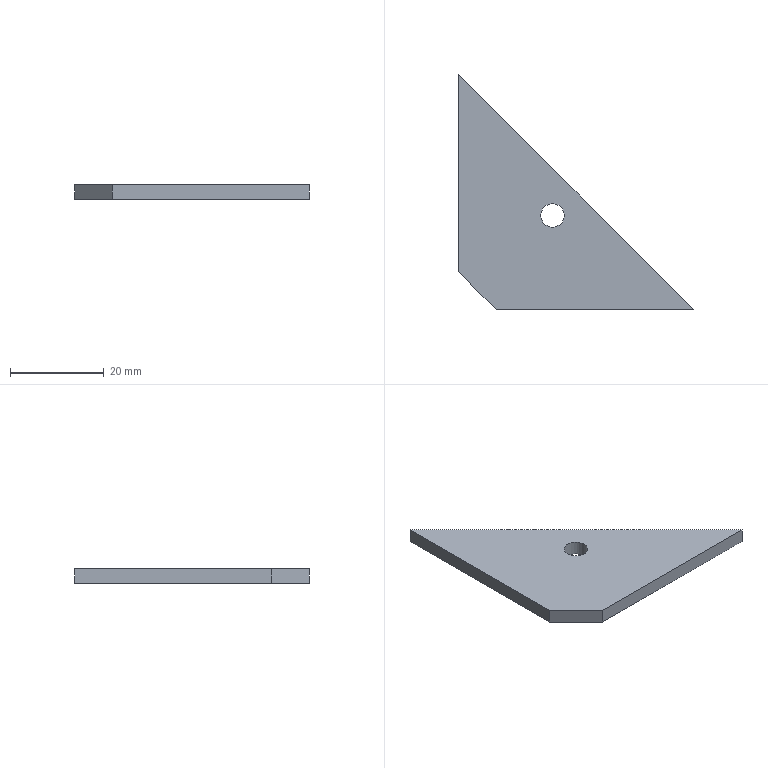Part | NX | 1 solid | 7 faces | box 50 x 50 x 3 mm | volume 3595 mm3 | plane 6 | cylinder 1 | commonest cylinder face diameters 5 x1
STEP:
#1=CARTESIAN_POINT('',(-17.,-25.,3.));
#2=VERTEX_POINT('',#1);
#3=CARTESIAN_POINT('',(25.,-25.,3.));
#4=VERTEX_POINT('',#3);
#5=CARTESIAN_POINT('',(-25.,-25.,3.));
#6=DIRECTION('',(1.,0.,0.));
#7=VECTOR('',#6,1000.);
#8=LINE('',#5,#7);
#9=EDGE_CURVE('',#2,#4,#8,.T.);
#10=ORIENTED_EDGE('',*,*,#9,.F.);
#11=CARTESIAN_POINT('',(-17.,-25.,0.));
#12=VERTEX_POINT('',#11);
#13=CARTESIAN_POINT('',(-17.,-25.,3.));
#14=DIRECTION('',(0.,0.,-1.));
#15=VECTOR('',#14,1000.);
#16=LINE('',#13,#15);
#17=EDGE_CURVE('',#2,#12,#16,.T.);
#18=ORIENTED_EDGE('',*,*,#17,.T.);
#19=CARTESIAN_POINT('',(25.,-25.,0.));
#20=VERTEX_POINT('',#19);
#21=CARTESIAN_POINT('',(-25.,-25.,0.));
#22=DIRECTION('',(1.,0.,0.));
#23=VECTOR('',#22,1000.);
#24=LINE('',#21,#23);
#25=EDGE_CURVE('',#12,#20,#24,.T.);
#26=ORIENTED_EDGE('',*,*,#25,.T.);
#27=CARTESIAN_POINT('',(25.,-25.,3.));
#28=DIRECTION('',(0.,0.,-1.));
#29=VECTOR('',#28,1000.);
#30=LINE('',#27,#29);
#31=EDGE_CURVE('',#4,#20,#30,.T.);
#32=ORIENTED_EDGE('',*,*,#31,.F.);
#33=EDGE_LOOP('',(#10,#18,#26,#32));
#34=FACE_BOUND('',#33,.T.);
#35=CARTESIAN_POINT('',(-25.,-25.,3.));
#36=DIRECTION('',(0.,1.,0.));
#37=DIRECTION('',(0.,0.,1.));
#38=AXIS2_PLACEMENT_3D('',#35,#36,#37);
#39=PLANE('',#38);
#40=ADVANCED_FACE('',(#34),#39,.F.);
#41=CARTESIAN_POINT('',(-25.,25.,0.));
#42=VERTEX_POINT('',#41);
#43=CARTESIAN_POINT('',(-25.,25.,0.));
#44=DIRECTION('',(-0.7071,0.7071,0.));
#45=VECTOR('',#44,1000.);
#46=LINE('',#43,#45);
#47=EDGE_CURVE('',#20,#42,#46,.T.);
#48=ORIENTED_EDGE('',*,*,#47,.T.);
#49=CARTESIAN_POINT('',(-25.,25.,3.));
#50=VERTEX_POINT('',#49);
#51=CARTESIAN_POINT('',(-25.,25.,3.));
#52=DIRECTION('',(0.,0.,-1.));
#53=VECTOR('',#52,1000.);
#54=LINE('',#51,#53);
#55=EDGE_CURVE('',#50,#42,#54,.T.);
#56=ORIENTED_EDGE('',*,*,#55,.F.);
#57=CARTESIAN_POINT('',(-25.,25.,3.));
#58=DIRECTION('',(-0.7071,0.7071,0.));
#59=VECTOR('',#58,1000.);
#60=LINE('',#57,#59);
#61=EDGE_CURVE('',#4,#50,#60,.T.);
#62=ORIENTED_EDGE('',*,*,#61,.F.);
#63=ORIENTED_EDGE('',*,*,#31,.T.);
#64=EDGE_LOOP('',(#48,#56,#62,#63));
#65=FACE_BOUND('',#64,.T.);
#66=CARTESIAN_POINT('',(-25.,25.,3.));
#67=DIRECTION('',(-0.7071,-0.7071,0.));
#68=DIRECTION('',(0.7071,-0.7071,0.));
#69=AXIS2_PLACEMENT_3D('',#66,#67,#68);
#70=PLANE('',#69);
#71=ADVANCED_FACE('',(#65),#70,.F.);
#72=CARTESIAN_POINT('',(-25.,-17.,0.));
#73=VERTEX_POINT('',#72);
#74=CARTESIAN_POINT('',(-25.,25.,0.));
#75=DIRECTION('',(0.,-1.,0.));
#76=VECTOR('',#75,1000.);
#77=LINE('',#74,#76);
#78=EDGE_CURVE('',#42,#73,#77,.T.);
#79=ORIENTED_EDGE('',*,*,#78,.T.);
#80=CARTESIAN_POINT('',(-25.,-17.,3.));
#81=VERTEX_POINT('',#80);
#82=CARTESIAN_POINT('',(-25.,-17.,3.));
#83=DIRECTION('',(0.,0.,1.));
#84=VECTOR('',#83,1000.);
#85=LINE('',#82,#84);
#86=EDGE_CURVE('',#73,#81,#85,.T.);
#87=ORIENTED_EDGE('',*,*,#86,.T.);
#88=CARTESIAN_POINT('',(-25.,25.,3.));
#89=DIRECTION('',(0.,-1.,0.));
#90=VECTOR('',#89,1000.);
#91=LINE('',#88,#90);
#92=EDGE_CURVE('',#50,#81,#91,.T.);
#93=ORIENTED_EDGE('',*,*,#92,.F.);
#94=ORIENTED_EDGE('',*,*,#55,.T.);
#95=EDGE_LOOP('',(#79,#87,#93,#94));
#96=FACE_BOUND('',#95,.T.);
#97=CARTESIAN_POINT('',(-25.,25.,3.));
#98=DIRECTION('',(1.,0.,0.));
#99=DIRECTION('',(0.,1.,0.));
#100=AXIS2_PLACEMENT_3D('',#97,#98,#99);
#101=PLANE('',#100);
#102=ADVANCED_FACE('',(#96),#101,.F.);
#103=CARTESIAN_POINT('',(-2.5,-5.,3.));
#104=VERTEX_POINT('',#103);
#105=CARTESIAN_POINT('',(-5.,-5.,3.));
#106=DIRECTION('',(0.,0.,1.));
#107=DIRECTION('',(1.,0.,0.));
#108=AXIS2_PLACEMENT_3D('',#105,#106,#107);
#109=CIRCLE('',#108,2.5);
#110=EDGE_CURVE('',#104,#104,#109,.T.);
#111=ORIENTED_EDGE('',*,*,#110,.F.);
#112=EDGE_LOOP('',(#111));
#113=FACE_BOUND('',#112,.T.);
#114=ORIENTED_EDGE('',*,*,#92,.T.);
#115=CARTESIAN_POINT('',(-17.,-25.,3.));
#116=DIRECTION('',(-0.7071,0.7071,0.));
#117=VECTOR('',#116,1000.);
#118=LINE('',#115,#117);
#119=EDGE_CURVE('',#81,#2,#118,.F.);
#120=ORIENTED_EDGE('',*,*,#119,.T.);
#121=ORIENTED_EDGE('',*,*,#9,.T.);
#122=ORIENTED_EDGE('',*,*,#61,.T.);
#123=EDGE_LOOP('',(#114,#120,#121,#122));
#124=FACE_BOUND('',#123,.T.);
#125=CARTESIAN_POINT('',(0.,0.,3.));
#126=DIRECTION('',(0.,0.,-1.));
#127=DIRECTION('',(-1.,0.,0.));
#128=AXIS2_PLACEMENT_3D('',#125,#126,#127);
#129=PLANE('',#128);
#130=ADVANCED_FACE('',(#113,#124),#129,.F.);
#131=CARTESIAN_POINT('',(-2.5,-5.,0.));
#132=VERTEX_POINT('',#131);
#133=CARTESIAN_POINT('',(-5.,-5.,0.));
#134=DIRECTION('',(0.,0.,1.));
#135=DIRECTION('',(1.,0.,0.));
#136=AXIS2_PLACEMENT_3D('',#133,#134,#135);
#137=CIRCLE('',#136,2.5);
#138=EDGE_CURVE('',#132,#132,#137,.T.);
#139=ORIENTED_EDGE('',*,*,#138,.T.);
#140=EDGE_LOOP('',(#139));
#141=FACE_BOUND('',#140,.T.);
#142=ORIENTED_EDGE('',*,*,#25,.F.);
#143=CARTESIAN_POINT('',(-21.,-21.,0.));
#144=DIRECTION('',(0.7071,-0.7071,0.));
#145=VECTOR('',#144,1000.);
#146=LINE('',#143,#145);
#147=EDGE_CURVE('',#12,#73,#146,.F.);
#148=ORIENTED_EDGE('',*,*,#147,.T.);
#149=ORIENTED_EDGE('',*,*,#78,.F.);
#150=ORIENTED_EDGE('',*,*,#47,.F.);
#151=EDGE_LOOP('',(#142,#148,#149,#150));
#152=FACE_BOUND('',#151,.T.);
#153=CARTESIAN_POINT('',(0.,0.,0.));
#154=DIRECTION('',(0.,0.,-1.));
#155=DIRECTION('',(-1.,0.,0.));
#156=AXIS2_PLACEMENT_3D('',#153,#154,#155);
#157=PLANE('',#156);
#158=ADVANCED_FACE('',(#141,#152),#157,.T.);
#159=ORIENTED_EDGE('',*,*,#119,.F.);
#160=ORIENTED_EDGE('',*,*,#86,.F.);
#161=ORIENTED_EDGE('',*,*,#147,.F.);
#162=ORIENTED_EDGE('',*,*,#17,.F.);
#163=EDGE_LOOP('',(#159,#160,#161,#162));
#164=FACE_BOUND('',#163,.T.);
#165=CARTESIAN_POINT('',(-17.,-25.,3.));
#166=DIRECTION('',(0.7071,0.7071,0.));
#167=DIRECTION('',(0.,0.,-1.));
#168=AXIS2_PLACEMENT_3D('',#165,#166,#167);
#169=PLANE('',#168);
#170=ADVANCED_FACE('',(#164),#169,.F.);
#171=ORIENTED_EDGE('',*,*,#138,.F.);
#172=EDGE_LOOP('',(#171));
#173=FACE_BOUND('',#172,.T.);
#174=ORIENTED_EDGE('',*,*,#110,.T.);
#175=EDGE_LOOP('',(#174));
#176=FACE_BOUND('',#175,.T.);
#177=CARTESIAN_POINT('',(-5.,-5.,3.));
#178=DIRECTION('',(0.,0.,1.));
#179=DIRECTION('',(1.,0.,0.));
#180=AXIS2_PLACEMENT_3D('',#177,#178,#179);
#181=CYLINDRICAL_SURFACE('',#180,2.5);
#182=ADVANCED_FACE('',(#173,#176),#181,.F.);
#183=CLOSED_SHELL('',(#40,#71,#102,#130,#158,#170,#182));
#184=MANIFOLD_SOLID_BREP('',#183);
#185=(LENGTH_UNIT()NAMED_UNIT(*)SI_UNIT(.MILLI.,.METRE.));
#186=UNCERTAINTY_MEASURE_WITH_UNIT(LENGTH_MEASURE(0.00001),#185,'','');
#187=(NAMED_UNIT(*)PLANE_ANGLE_UNIT()SI_UNIT($,.RADIAN.));
#188=(NAMED_UNIT(*)SI_UNIT($,.STERADIAN.)SOLID_ANGLE_UNIT());
#189=(GEOMETRIC_REPRESENTATION_CONTEXT(3)GLOBAL_UNCERTAINTY_ASSIGNED_CONTEXT((#186))GLOBAL_UNIT_ASSIGNED_CONTEXT((#185,#187,#188))REPRESENTATION_CONTEXT('',''));
#190=ADVANCED_BREP_SHAPE_REPRESENTATION('',(#184),#189);